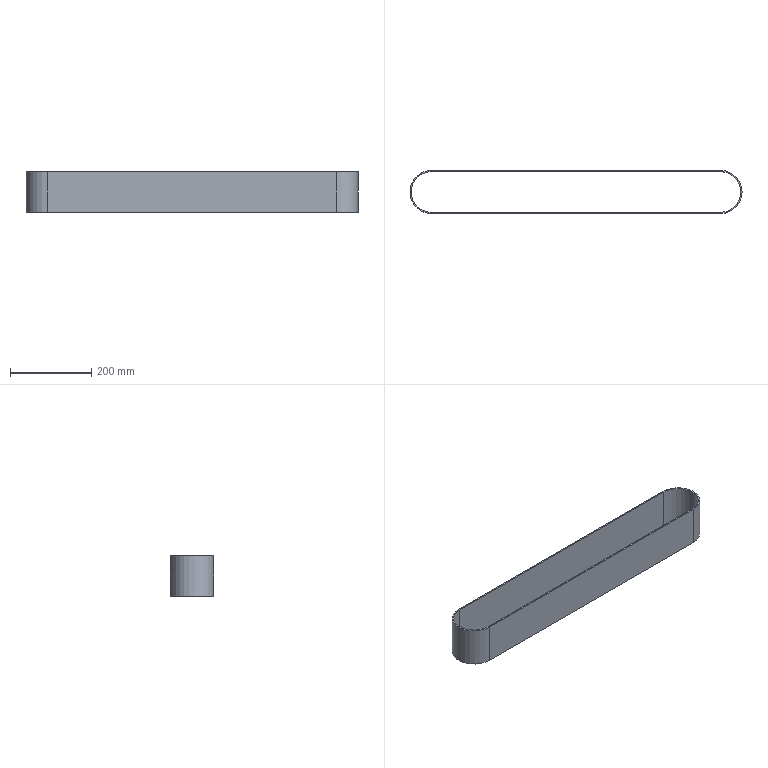Part | STEP file | 1 solid | 12 faces | box 816 x 106 x 100 mm | volume 523075 mm3 | cylinder 6 | plane 6 | commonest cylinder face diameters 100 x3 106 x3
STEP:
#1=CARTESIAN_POINT('',(0.,0.,0.));
#2=DIRECTION('',(0.,0.,1.));
#3=DIRECTION('',(1.,0.,0.));
#4=AXIS2_PLACEMENT_3D('',#1,#2,#3);
#5=CARTESIAN_POINT('',(550.53,56.408,0.));
#6=VERTEX_POINT('',#5);
#7=CARTESIAN_POINT('',(550.53,56.408,100.));
#8=VERTEX_POINT('',#7);
#9=CARTESIAN_POINT('',(550.53,56.408,0.));
#10=DIRECTION('',(0.,0.,1.));
#11=VECTOR('',#10,1.);
#12=LINE('',#9,#11);
#13=CARTESIAN_POINT('',(550.53,6.408,0.));
#14=DIRECTION('',(0.,0.,1.));
#15=DIRECTION('',(1.,0.,0.));
#16=AXIS2_PLACEMENT_3D('',#13,#14,#15);
#17=CYLINDRICAL_SURFACE('',#16,50.);
#18=CARTESIAN_POINT('',(1.571,0.));
#19=DIRECTION('',(0.,1.));
#20=VECTOR('',#19,1.);
#21=LINE('',#18,#20);
#22=(GEOMETRIC_REPRESENTATION_CONTEXT(2)PARAMETRIC_REPRESENTATION_CONTEXT()REPRESENTATION_CONTEXT('',''));
#23=DEFINITIONAL_REPRESENTATION('',(#21),#22);
#24=PCURVE('',#17,#23);
#25=CARTESIAN_POINT('',(550.53,56.408,0.));
#26=DIRECTION('',(0.,1.,0.));
#27=DIRECTION('',(-1.,0.,0.));
#28=AXIS2_PLACEMENT_3D('',#25,#26,#27);
#29=PLANE('',#28);
#30=CARTESIAN_POINT('',(0.,0.));
#31=DIRECTION('',(0.,1.));
#32=VECTOR('',#31,1.);
#33=LINE('',#30,#32);
#34=(GEOMETRIC_REPRESENTATION_CONTEXT(2)PARAMETRIC_REPRESENTATION_CONTEXT()REPRESENTATION_CONTEXT('',''));
#35=DEFINITIONAL_REPRESENTATION('',(#33),#34);
#36=PCURVE('',#29,#35);
#37=SURFACE_CURVE('',#12,(#24,#36),.PCURVE_S1.);
#38=EDGE_CURVE('',#6,#8,#37,.T.);
#39=ORIENTED_EDGE('',*,*,#38,.T.);
#40=CARTESIAN_POINT('',(600.53,6.408,100.));
#41=VERTEX_POINT('',#40);
#42=CARTESIAN_POINT('',(550.53,6.408,100.));
#43=DIRECTION('',(0.,0.,-1.));
#44=DIRECTION('',(1.,0.,0.));
#45=AXIS2_PLACEMENT_3D('',#42,#43,#44);
#46=CIRCLE('',#45,50.);
#47=CARTESIAN_POINT('',(6.283,100.));
#48=DIRECTION('',(-1.,0.));
#49=VECTOR('',#48,1.);
#50=LINE('',#47,#49);
#51=(GEOMETRIC_REPRESENTATION_CONTEXT(2)PARAMETRIC_REPRESENTATION_CONTEXT()REPRESENTATION_CONTEXT('',''));
#52=DEFINITIONAL_REPRESENTATION('',(#50),#51);
#53=PCURVE('',#17,#52);
#54=CARTESIAN_POINT('',(195.531,6.408,100.));
#55=DIRECTION('',(0.,0.,1.));
#56=DIRECTION('',(1.,0.,0.));
#57=AXIS2_PLACEMENT_3D('',#54,#55,#56);
#58=PLANE('',#57);
#59=CARTESIAN_POINT('',(405.,0.));
#60=CARTESIAN_POINT('',(405.,-86.603));
#61=CARTESIAN_POINT('',(330.,-43.301));
#62=CARTESIAN_POINT('',(255.,0.));
#63=CARTESIAN_POINT('',(330.,43.301));
#64=CARTESIAN_POINT('',(405.,86.603));
#65=CARTESIAN_POINT('',(405.,0.));
#66=(BOUNDED_CURVE()B_SPLINE_CURVE(2,(#59,#60,#61,#62,#63,#64,#65),.UNSPECIFIED.,.T.,.F.)B_SPLINE_CURVE_WITH_KNOTS((1,2,2,2,2,1),(-2.094,0.,2.094,4.189,6.283,8.378),.UNSPECIFIED.)CURVE()GEOMETRIC_REPRESENTATION_ITEM()RATIONAL_B_SPLINE_CURVE((1.,0.5,1.,0.5,1.,0.5,1.))REPRESENTATION_ITEM(''));
#67=(GEOMETRIC_REPRESENTATION_CONTEXT(2)PARAMETRIC_REPRESENTATION_CONTEXT()REPRESENTATION_CONTEXT('',''));
#68=DEFINITIONAL_REPRESENTATION('',(#66),#67);
#69=PCURVE('',#58,#68);
#70=SURFACE_CURVE('',#46,(#53,#69),.PCURVE_S1.);
#71=EDGE_CURVE('',#8,#41,#70,.T.);
#72=ORIENTED_EDGE('',*,*,#71,.T.);
#73=CARTESIAN_POINT('',(600.53,6.408,0.));
#74=VERTEX_POINT('',#73);
#75=CARTESIAN_POINT('',(600.53,6.408,0.));
#76=DIRECTION('',(0.,0.,1.));
#77=VECTOR('',#76,1.);
#78=LINE('',#75,#77);
#79=CARTESIAN_POINT('',(0.,0.));
#80=DIRECTION('',(0.,1.));
#81=VECTOR('',#80,1.);
#82=LINE('',#79,#81);
#83=(GEOMETRIC_REPRESENTATION_CONTEXT(2)PARAMETRIC_REPRESENTATION_CONTEXT()REPRESENTATION_CONTEXT('',''));
#84=DEFINITIONAL_REPRESENTATION('',(#82),#83);
#85=PCURVE('',#17,#84);
#86=CARTESIAN_POINT('',(550.53,6.408,0.));
#87=DIRECTION('',(0.,0.,1.));
#88=DIRECTION('',(1.,0.,0.));
#89=AXIS2_PLACEMENT_3D('',#86,#87,#88);
#90=CYLINDRICAL_SURFACE('',#89,50.);
#91=CARTESIAN_POINT('',(6.283,0.));
#92=DIRECTION('',(0.,1.));
#93=VECTOR('',#92,1.);
#94=LINE('',#91,#93);
#95=(GEOMETRIC_REPRESENTATION_CONTEXT(2)PARAMETRIC_REPRESENTATION_CONTEXT()REPRESENTATION_CONTEXT('',''));
#96=DEFINITIONAL_REPRESENTATION('',(#94),#95);
#97=PCURVE('',#90,#96);
#98=SURFACE_CURVE('',#78,(#85,#97),.PCURVE_S1.);
#99=EDGE_CURVE('',#74,#41,#98,.T.);
#100=ORIENTED_EDGE('',*,*,#99,.F.);
#101=CARTESIAN_POINT('',(550.53,6.408,0.));
#102=DIRECTION('',(0.,0.,-1.));
#103=DIRECTION('',(1.,0.,0.));
#104=AXIS2_PLACEMENT_3D('',#101,#102,#103);
#105=CIRCLE('',#104,50.);
#106=CARTESIAN_POINT('',(6.283,0.));
#107=DIRECTION('',(-1.,0.));
#108=VECTOR('',#107,1.);
#109=LINE('',#106,#108);
#110=(GEOMETRIC_REPRESENTATION_CONTEXT(2)PARAMETRIC_REPRESENTATION_CONTEXT()REPRESENTATION_CONTEXT('',''));
#111=DEFINITIONAL_REPRESENTATION('',(#109),#110);
#112=PCURVE('',#17,#111);
#113=CARTESIAN_POINT('',(195.531,6.408,0.));
#114=DIRECTION('',(0.,0.,1.));
#115=DIRECTION('',(1.,0.,0.));
#116=AXIS2_PLACEMENT_3D('',#113,#114,#115);
#117=PLANE('',#116);
#118=CARTESIAN_POINT('',(405.,0.));
#119=CARTESIAN_POINT('',(405.,-86.603));
#120=CARTESIAN_POINT('',(330.,-43.301));
#121=CARTESIAN_POINT('',(255.,0.));
#122=CARTESIAN_POINT('',(330.,43.301));
#123=CARTESIAN_POINT('',(405.,86.603));
#124=CARTESIAN_POINT('',(405.,0.));
#125=(BOUNDED_CURVE()B_SPLINE_CURVE(2,(#118,#119,#120,#121,#122,#123,#124),.UNSPECIFIED.,.T.,.F.)B_SPLINE_CURVE_WITH_KNOTS((1,2,2,2,2,1),(-2.094,0.,2.094,4.189,6.283,8.378),.UNSPECIFIED.)CURVE()GEOMETRIC_REPRESENTATION_ITEM()RATIONAL_B_SPLINE_CURVE((1.,0.5,1.,0.5,1.,0.5,1.))REPRESENTATION_ITEM(''));
#126=(GEOMETRIC_REPRESENTATION_CONTEXT(2)PARAMETRIC_REPRESENTATION_CONTEXT()REPRESENTATION_CONTEXT('',''));
#127=DEFINITIONAL_REPRESENTATION('',(#125),#126);
#128=PCURVE('',#117,#127);
#129=SURFACE_CURVE('',#105,(#112,#128),.PCURVE_S1.);
#130=EDGE_CURVE('',#6,#74,#129,.T.);
#131=ORIENTED_EDGE('',*,*,#130,.F.);
#132=EDGE_LOOP('',(#39,#72,#100,#131));
#133=FACE_BOUND('',#132,.F.);
#134=ADVANCED_FACE('',(#133),#17,.F.);
#135=CARTESIAN_POINT('',(550.53,-46.592,0.));
#136=VERTEX_POINT('',#135);
#137=CARTESIAN_POINT('',(603.53,6.408,0.));
#138=VERTEX_POINT('',#137);
#139=CARTESIAN_POINT('',(550.53,6.408,0.));
#140=DIRECTION('',(0.,0.,1.));
#141=DIRECTION('',(1.,0.,0.));
#142=AXIS2_PLACEMENT_3D('',#139,#140,#141);
#143=CIRCLE('',#142,53.);
#144=CARTESIAN_POINT('',(550.53,6.408,0.));
#145=DIRECTION('',(0.,0.,1.));
#146=DIRECTION('',(1.,0.,0.));
#147=AXIS2_PLACEMENT_3D('',#144,#145,#146);
#148=CYLINDRICAL_SURFACE('',#147,53.);
#149=CARTESIAN_POINT('',(0.,0.));
#150=DIRECTION('',(1.,0.));
#151=VECTOR('',#150,1.);
#152=LINE('',#149,#151);
#153=(GEOMETRIC_REPRESENTATION_CONTEXT(2)PARAMETRIC_REPRESENTATION_CONTEXT()REPRESENTATION_CONTEXT('',''));
#154=DEFINITIONAL_REPRESENTATION('',(#152),#153);
#155=PCURVE('',#148,#154);
#156=CARTESIAN_POINT('',(355.,0.));
#157=DIRECTION('',(1.,0.));
#158=AXIS2_PLACEMENT_2D('',#156,#157);
#159=CIRCLE('',#158,53.);
#160=(GEOMETRIC_REPRESENTATION_CONTEXT(2)PARAMETRIC_REPRESENTATION_CONTEXT()REPRESENTATION_CONTEXT('',''));
#161=DEFINITIONAL_REPRESENTATION('',(#159),#160);
#162=PCURVE('',#117,#161);
#163=SURFACE_CURVE('',#143,(#155,#162),.PCURVE_S1.);
#164=EDGE_CURVE('',#136,#138,#163,.T.);
#165=ORIENTED_EDGE('',*,*,#164,.T.);
#166=CARTESIAN_POINT('',(603.53,6.408,100.));
#167=VERTEX_POINT('',#166);
#168=CARTESIAN_POINT('',(603.53,6.408,0.));
#169=DIRECTION('',(0.,0.,1.));
#170=VECTOR('',#169,1.);
#171=LINE('',#168,#170);
#172=CARTESIAN_POINT('',(6.283,0.));
#173=DIRECTION('',(0.,1.));
#174=VECTOR('',#173,1.);
#175=LINE('',#172,#174);
#176=(GEOMETRIC_REPRESENTATION_CONTEXT(2)PARAMETRIC_REPRESENTATION_CONTEXT()REPRESENTATION_CONTEXT('',''));
#177=DEFINITIONAL_REPRESENTATION('',(#175),#176);
#178=PCURVE('',#148,#177);
#179=CARTESIAN_POINT('',(550.53,6.408,0.));
#180=DIRECTION('',(0.,0.,1.));
#181=DIRECTION('',(1.,0.,0.));
#182=AXIS2_PLACEMENT_3D('',#179,#180,#181);
#183=CYLINDRICAL_SURFACE('',#182,53.);
#184=CARTESIAN_POINT('',(0.,0.));
#185=DIRECTION('',(0.,1.));
#186=VECTOR('',#185,1.);
#187=LINE('',#184,#186);
#188=(GEOMETRIC_REPRESENTATION_CONTEXT(2)PARAMETRIC_REPRESENTATION_CONTEXT()REPRESENTATION_CONTEXT('',''));
#189=DEFINITIONAL_REPRESENTATION('',(#187),#188);
#190=PCURVE('',#183,#189);
#191=SURFACE_CURVE('',#171,(#178,#190),.PCURVE_S1.);
#192=EDGE_CURVE('',#138,#167,#191,.T.);
#193=ORIENTED_EDGE('',*,*,#192,.T.);
#194=CARTESIAN_POINT('',(550.53,-46.592,100.));
#195=VERTEX_POINT('',#194);
#196=CARTESIAN_POINT('',(550.53,6.408,100.));
#197=DIRECTION('',(0.,0.,1.));
#198=DIRECTION('',(1.,0.,0.));
#199=AXIS2_PLACEMENT_3D('',#196,#197,#198);
#200=CIRCLE('',#199,53.);
#201=CARTESIAN_POINT('',(0.,100.));
#202=DIRECTION('',(1.,0.));
#203=VECTOR('',#202,1.);
#204=LINE('',#201,#203);
#205=(GEOMETRIC_REPRESENTATION_CONTEXT(2)PARAMETRIC_REPRESENTATION_CONTEXT()REPRESENTATION_CONTEXT('',''));
#206=DEFINITIONAL_REPRESENTATION('',(#204),#205);
#207=PCURVE('',#148,#206);
#208=CARTESIAN_POINT('',(355.,0.));
#209=DIRECTION('',(1.,0.));
#210=AXIS2_PLACEMENT_2D('',#208,#209);
#211=CIRCLE('',#210,53.);
#212=(GEOMETRIC_REPRESENTATION_CONTEXT(2)PARAMETRIC_REPRESENTATION_CONTEXT()REPRESENTATION_CONTEXT('',''));
#213=DEFINITIONAL_REPRESENTATION('',(#211),#212);
#214=PCURVE('',#58,#213);
#215=SURFACE_CURVE('',#200,(#207,#214),.PCURVE_S1.);
#216=EDGE_CURVE('',#195,#167,#215,.T.);
#217=ORIENTED_EDGE('',*,*,#216,.F.);
#218=CARTESIAN_POINT('',(550.53,-46.592,0.));
#219=DIRECTION('',(0.,0.,-1.));
#220=VECTOR('',#219,1.);
#221=LINE('',#218,#220);
#222=CARTESIAN_POINT('',(4.712,0.));
#223=DIRECTION('',(0.,-1.));
#224=VECTOR('',#223,1.);
#225=LINE('',#222,#224);
#226=(GEOMETRIC_REPRESENTATION_CONTEXT(2)PARAMETRIC_REPRESENTATION_CONTEXT()REPRESENTATION_CONTEXT('',''));
#227=DEFINITIONAL_REPRESENTATION('',(#225),#226);
#228=PCURVE('',#148,#227);
#229=CARTESIAN_POINT('',(-159.47,-46.592,0.));
#230=DIRECTION('',(0.,-1.,0.));
#231=DIRECTION('',(1.,0.,0.));
#232=AXIS2_PLACEMENT_3D('',#229,#230,#231);
#233=PLANE('',#232);
#234=CARTESIAN_POINT('',(710.,0.));
#235=DIRECTION('',(0.,-1.));
#236=VECTOR('',#235,1.);
#237=LINE('',#234,#236);
#238=(GEOMETRIC_REPRESENTATION_CONTEXT(2)PARAMETRIC_REPRESENTATION_CONTEXT()REPRESENTATION_CONTEXT('',''));
#239=DEFINITIONAL_REPRESENTATION('',(#237),#238);
#240=PCURVE('',#233,#239);
#241=SURFACE_CURVE('',#221,(#228,#240),.PCURVE_S1.);
#242=EDGE_CURVE('',#195,#136,#241,.T.);
#243=ORIENTED_EDGE('',*,*,#242,.T.);
#244=EDGE_LOOP('',(#165,#193,#217,#243));
#245=FACE_BOUND('',#244,.T.);
#246=ADVANCED_FACE('',(#245),#148,.T.);
#247=CARTESIAN_POINT('',(-159.47,-43.592,100.));
#248=VERTEX_POINT('',#247);
#249=CARTESIAN_POINT('',(-159.47,-43.592,0.));
#250=VERTEX_POINT('',#249);
#251=CARTESIAN_POINT('',(-159.47,-43.592,0.));
#252=DIRECTION('',(0.,0.,-1.));
#253=VECTOR('',#252,1.);
#254=LINE('',#251,#253);
#255=CARTESIAN_POINT('',(-159.47,-43.592,0.));
#256=DIRECTION('',(0.,-1.,0.));
#257=DIRECTION('',(1.,0.,0.));
#258=AXIS2_PLACEMENT_3D('',#255,#256,#257);
#259=PLANE('',#258);
#260=CARTESIAN_POINT('',(0.,0.));
#261=DIRECTION('',(0.,-1.));
#262=VECTOR('',#261,1.);
#263=LINE('',#260,#262);
#264=(GEOMETRIC_REPRESENTATION_CONTEXT(2)PARAMETRIC_REPRESENTATION_CONTEXT()REPRESENTATION_CONTEXT('',''));
#265=DEFINITIONAL_REPRESENTATION('',(#263),#264);
#266=PCURVE('',#259,#265);
#267=CARTESIAN_POINT('',(-159.47,6.408,0.));
#268=DIRECTION('',(0.,0.,1.));
#269=DIRECTION('',(1.,0.,0.));
#270=AXIS2_PLACEMENT_3D('',#267,#268,#269);
#271=CYLINDRICAL_SURFACE('',#270,50.);
#272=CARTESIAN_POINT('',(4.712,0.));
#273=DIRECTION('',(0.,-1.));
#274=VECTOR('',#273,1.);
#275=LINE('',#272,#274);
#276=(GEOMETRIC_REPRESENTATION_CONTEXT(2)PARAMETRIC_REPRESENTATION_CONTEXT()REPRESENTATION_CONTEXT('',''));
#277=DEFINITIONAL_REPRESENTATION('',(#275),#276);
#278=PCURVE('',#271,#277);
#279=SURFACE_CURVE('',#254,(#266,#278),.PCURVE_S1.);
#280=EDGE_CURVE('',#248,#250,#279,.T.);
#281=ORIENTED_EDGE('',*,*,#280,.F.);
#282=CARTESIAN_POINT('',(550.53,-43.592,100.));
#283=VERTEX_POINT('',#282);
#284=CARTESIAN_POINT('',(-159.47,-43.592,100.));
#285=DIRECTION('',(-1.,0.,0.));
#286=VECTOR('',#285,1.);
#287=LINE('',#284,#286);
#288=CARTESIAN_POINT('',(0.,100.));
#289=DIRECTION('',(-1.,0.));
#290=VECTOR('',#289,1.);
#291=LINE('',#288,#290);
#292=(GEOMETRIC_REPRESENTATION_CONTEXT(2)PARAMETRIC_REPRESENTATION_CONTEXT()REPRESENTATION_CONTEXT('',''));
#293=DEFINITIONAL_REPRESENTATION('',(#291),#292);
#294=PCURVE('',#259,#293);
#295=CARTESIAN_POINT('',(-355.,-50.));
#296=DIRECTION('',(-1.,0.));
#297=VECTOR('',#296,1.);
#298=LINE('',#295,#297);
#299=(GEOMETRIC_REPRESENTATION_CONTEXT(2)PARAMETRIC_REPRESENTATION_CONTEXT()REPRESENTATION_CONTEXT('',''));
#300=DEFINITIONAL_REPRESENTATION('',(#298),#299);
#301=PCURVE('',#58,#300);
#302=SURFACE_CURVE('',#287,(#294,#301),.PCURVE_S1.);
#303=EDGE_CURVE('',#283,#248,#302,.T.);
#304=ORIENTED_EDGE('',*,*,#303,.F.);
#305=CARTESIAN_POINT('',(550.53,-43.592,0.));
#306=VERTEX_POINT('',#305);
#307=CARTESIAN_POINT('',(550.53,-43.592,0.));
#308=DIRECTION('',(0.,0.,1.));
#309=VECTOR('',#308,1.);
#310=LINE('',#307,#309);
#311=CARTESIAN_POINT('',(710.,0.));
#312=DIRECTION('',(0.,1.));
#313=VECTOR('',#312,1.);
#314=LINE('',#311,#313);
#315=(GEOMETRIC_REPRESENTATION_CONTEXT(2)PARAMETRIC_REPRESENTATION_CONTEXT()REPRESENTATION_CONTEXT('',''));
#316=DEFINITIONAL_REPRESENTATION('',(#314),#315);
#317=PCURVE('',#259,#316);
#318=CARTESIAN_POINT('',(4.712,0.));
#319=DIRECTION('',(0.,1.));
#320=VECTOR('',#319,1.);
#321=LINE('',#318,#320);
#322=(GEOMETRIC_REPRESENTATION_CONTEXT(2)PARAMETRIC_REPRESENTATION_CONTEXT()REPRESENTATION_CONTEXT('',''));
#323=DEFINITIONAL_REPRESENTATION('',(#321),#322);
#324=PCURVE('',#90,#323);
#325=SURFACE_CURVE('',#310,(#317,#324),.PCURVE_S1.);
#326=EDGE_CURVE('',#306,#283,#325,.T.);
#327=ORIENTED_EDGE('',*,*,#326,.F.);
#328=CARTESIAN_POINT('',(-159.47,-43.592,0.));
#329=DIRECTION('',(1.,0.,0.));
#330=VECTOR('',#329,1.);
#331=LINE('',#328,#330);
#332=CARTESIAN_POINT('',(0.,0.));
#333=DIRECTION('',(1.,0.));
#334=VECTOR('',#333,1.);
#335=LINE('',#332,#334);
#336=(GEOMETRIC_REPRESENTATION_CONTEXT(2)PARAMETRIC_REPRESENTATION_CONTEXT()REPRESENTATION_CONTEXT('',''));
#337=DEFINITIONAL_REPRESENTATION('',(#335),#336);
#338=PCURVE('',#259,#337);
#339=CARTESIAN_POINT('',(-355.,-50.));
#340=DIRECTION('',(1.,0.));
#341=VECTOR('',#340,1.);
#342=LINE('',#339,#341);
#343=(GEOMETRIC_REPRESENTATION_CONTEXT(2)PARAMETRIC_REPRESENTATION_CONTEXT()REPRESENTATION_CONTEXT('',''));
#344=DEFINITIONAL_REPRESENTATION('',(#342),#343);
#345=PCURVE('',#117,#344);
#346=SURFACE_CURVE('',#331,(#338,#345),.PCURVE_S1.);
#347=EDGE_CURVE('',#250,#306,#346,.T.);
#348=ORIENTED_EDGE('',*,*,#347,.F.);
#349=EDGE_LOOP('',(#281,#304,#327,#348));
#350=FACE_BOUND('',#349,.T.);
#351=ADVANCED_FACE('',(#350),#259,.F.);
#352=ORIENTED_EDGE('',*,*,#164,.F.);
#353=CARTESIAN_POINT('',(-159.47,-46.592,0.));
#354=VERTEX_POINT('',#353);
#355=CARTESIAN_POINT('',(195.531,-46.592,0.));
#356=DIRECTION('',(1.,0.,0.));
#357=VECTOR('',#356,1.);
#358=LINE('',#355,#357);
#359=CARTESIAN_POINT('',(0.,-53.));
#360=DIRECTION('',(1.,0.));
#361=VECTOR('',#360,1.);
#362=LINE('',#359,#361);
#363=(GEOMETRIC_REPRESENTATION_CONTEXT(2)PARAMETRIC_REPRESENTATION_CONTEXT()REPRESENTATION_CONTEXT('',''));
#364=DEFINITIONAL_REPRESENTATION('',(#362),#363);
#365=PCURVE('',#117,#364);
#366=CARTESIAN_POINT('',(355.,0.));
#367=DIRECTION('',(1.,0.));
#368=VECTOR('',#367,1.);
#369=LINE('',#366,#368);
#370=(GEOMETRIC_REPRESENTATION_CONTEXT(2)PARAMETRIC_REPRESENTATION_CONTEXT()REPRESENTATION_CONTEXT('',''));
#371=DEFINITIONAL_REPRESENTATION('',(#369),#370);
#372=PCURVE('',#233,#371);
#373=SURFACE_CURVE('',#358,(#365,#372),.PCURVE_S1.);
#374=EDGE_CURVE('',#354,#136,#373,.T.);
#375=ORIENTED_EDGE('',*,*,#374,.F.);
#376=CARTESIAN_POINT('',(-159.47,59.408,0.));
#377=VERTEX_POINT('',#376);
#378=CARTESIAN_POINT('',(-159.47,6.408,0.));
#379=DIRECTION('',(0.,0.,1.));
#380=DIRECTION('',(1.,0.,0.));
#381=AXIS2_PLACEMENT_3D('',#378,#379,#380);
#382=CIRCLE('',#381,53.);
#383=CARTESIAN_POINT('',(-355.,0.));
#384=DIRECTION('',(1.,0.));
#385=AXIS2_PLACEMENT_2D('',#383,#384);
#386=CIRCLE('',#385,53.);
#387=(GEOMETRIC_REPRESENTATION_CONTEXT(2)PARAMETRIC_REPRESENTATION_CONTEXT()REPRESENTATION_CONTEXT('',''));
#388=DEFINITIONAL_REPRESENTATION('',(#386),#387);
#389=PCURVE('',#117,#388);
#390=CARTESIAN_POINT('',(-159.47,6.408,0.));
#391=DIRECTION('',(0.,0.,1.));
#392=DIRECTION('',(1.,0.,0.));
#393=AXIS2_PLACEMENT_3D('',#390,#391,#392);
#394=CYLINDRICAL_SURFACE('',#393,53.);
#395=CARTESIAN_POINT('',(0.,0.));
#396=DIRECTION('',(1.,0.));
#397=VECTOR('',#396,1.);
#398=LINE('',#395,#397);
#399=(GEOMETRIC_REPRESENTATION_CONTEXT(2)PARAMETRIC_REPRESENTATION_CONTEXT()REPRESENTATION_CONTEXT('',''));
#400=DEFINITIONAL_REPRESENTATION('',(#398),#399);
#401=PCURVE('',#394,#400);
#402=SURFACE_CURVE('',#382,(#389,#401),.PCURVE_S1.);
#403=EDGE_CURVE('',#377,#354,#402,.T.);
#404=ORIENTED_EDGE('',*,*,#403,.F.);
#405=CARTESIAN_POINT('',(550.53,59.408,0.));
#406=VERTEX_POINT('',#405);
#407=CARTESIAN_POINT('',(195.531,59.408,0.));
#408=DIRECTION('',(-1.,0.,0.));
#409=VECTOR('',#408,1.);
#410=LINE('',#407,#409);
#411=CARTESIAN_POINT('',(0.,53.));
#412=DIRECTION('',(-1.,0.));
#413=VECTOR('',#412,1.);
#414=LINE('',#411,#413);
#415=(GEOMETRIC_REPRESENTATION_CONTEXT(2)PARAMETRIC_REPRESENTATION_CONTEXT()REPRESENTATION_CONTEXT('',''));
#416=DEFINITIONAL_REPRESENTATION('',(#414),#415);
#417=PCURVE('',#117,#416);
#418=CARTESIAN_POINT('',(550.53,59.408,0.));
#419=DIRECTION('',(0.,1.,0.));
#420=DIRECTION('',(-1.,0.,0.));
#421=AXIS2_PLACEMENT_3D('',#418,#419,#420);
#422=PLANE('',#421);
#423=CARTESIAN_POINT('',(355.,0.));
#424=DIRECTION('',(1.,0.));
#425=VECTOR('',#424,1.);
#426=LINE('',#423,#425);
#427=(GEOMETRIC_REPRESENTATION_CONTEXT(2)PARAMETRIC_REPRESENTATION_CONTEXT()REPRESENTATION_CONTEXT('',''));
#428=DEFINITIONAL_REPRESENTATION('',(#426),#427);
#429=PCURVE('',#422,#428);
#430=SURFACE_CURVE('',#410,(#417,#429),.PCURVE_S1.);
#431=EDGE_CURVE('',#406,#377,#430,.T.);
#432=ORIENTED_EDGE('',*,*,#431,.F.);
#433=CARTESIAN_POINT('',(550.53,6.408,0.));
#434=DIRECTION('',(0.,0.,1.));
#435=DIRECTION('',(1.,0.,0.));
#436=AXIS2_PLACEMENT_3D('',#433,#434,#435);
#437=CIRCLE('',#436,53.);
#438=CARTESIAN_POINT('',(355.,0.));
#439=DIRECTION('',(1.,0.));
#440=AXIS2_PLACEMENT_2D('',#438,#439);
#441=CIRCLE('',#440,53.);
#442=(GEOMETRIC_REPRESENTATION_CONTEXT(2)PARAMETRIC_REPRESENTATION_CONTEXT()REPRESENTATION_CONTEXT('',''));
#443=DEFINITIONAL_REPRESENTATION('',(#441),#442);
#444=PCURVE('',#117,#443);
#445=CARTESIAN_POINT('',(0.,0.));
#446=DIRECTION('',(1.,0.));
#447=VECTOR('',#446,1.);
#448=LINE('',#445,#447);
#449=(GEOMETRIC_REPRESENTATION_CONTEXT(2)PARAMETRIC_REPRESENTATION_CONTEXT()REPRESENTATION_CONTEXT('',''));
#450=DEFINITIONAL_REPRESENTATION('',(#448),#449);
#451=PCURVE('',#183,#450);
#452=SURFACE_CURVE('',#437,(#444,#451),.PCURVE_S1.);
#453=EDGE_CURVE('',#138,#406,#452,.T.);
#454=ORIENTED_EDGE('',*,*,#453,.F.);
#455=EDGE_LOOP('',(#352,#375,#404,#432,#454));
#456=FACE_BOUND('',#455,.T.);
#457=CARTESIAN_POINT('',(-159.47,56.408,0.));
#458=VERTEX_POINT('',#457);
#459=CARTESIAN_POINT('',(195.531,56.408,0.));
#460=DIRECTION('',(1.,0.,0.));
#461=VECTOR('',#460,1.);
#462=LINE('',#459,#461);
#463=CARTESIAN_POINT('',(0.,50.));
#464=DIRECTION('',(1.,0.));
#465=VECTOR('',#464,1.);
#466=LINE('',#463,#465);
#467=(GEOMETRIC_REPRESENTATION_CONTEXT(2)PARAMETRIC_REPRESENTATION_CONTEXT()REPRESENTATION_CONTEXT('',''));
#468=DEFINITIONAL_REPRESENTATION('',(#466),#467);
#469=PCURVE('',#117,#468);
#470=CARTESIAN_POINT('',(355.,0.));
#471=DIRECTION('',(-1.,0.));
#472=VECTOR('',#471,1.);
#473=LINE('',#470,#472);
#474=(GEOMETRIC_REPRESENTATION_CONTEXT(2)PARAMETRIC_REPRESENTATION_CONTEXT()REPRESENTATION_CONTEXT('',''));
#475=DEFINITIONAL_REPRESENTATION('',(#473),#474);
#476=PCURVE('',#29,#475);
#477=SURFACE_CURVE('',#462,(#469,#476),.PCURVE_S1.);
#478=EDGE_CURVE('',#458,#6,#477,.T.);
#479=ORIENTED_EDGE('',*,*,#478,.F.);
#480=CARTESIAN_POINT('',(-159.47,6.408,0.));
#481=DIRECTION('',(0.,0.,-1.));
#482=DIRECTION('',(1.,0.,0.));
#483=AXIS2_PLACEMENT_3D('',#480,#481,#482);
#484=CIRCLE('',#483,50.);
#485=CARTESIAN_POINT('',(-305.,0.));
#486=CARTESIAN_POINT('',(-305.,-86.603));
#487=CARTESIAN_POINT('',(-380.,-43.301));
#488=CARTESIAN_POINT('',(-455.,0.));
#489=CARTESIAN_POINT('',(-380.,43.301));
#490=CARTESIAN_POINT('',(-305.,86.603));
#491=CARTESIAN_POINT('',(-305.,0.));
#492=(BOUNDED_CURVE()B_SPLINE_CURVE(2,(#485,#486,#487,#488,#489,#490,#491),.UNSPECIFIED.,.T.,.F.)B_SPLINE_CURVE_WITH_KNOTS((1,2,2,2,2,1),(-2.094,0.,2.094,4.189,6.283,8.378),.UNSPECIFIED.)CURVE()GEOMETRIC_REPRESENTATION_ITEM()RATIONAL_B_SPLINE_CURVE((1.,0.5,1.,0.5,1.,0.5,1.))REPRESENTATION_ITEM(''));
#493=(GEOMETRIC_REPRESENTATION_CONTEXT(2)PARAMETRIC_REPRESENTATION_CONTEXT()REPRESENTATION_CONTEXT('',''));
#494=DEFINITIONAL_REPRESENTATION('',(#492),#493);
#495=PCURVE('',#117,#494);
#496=CARTESIAN_POINT('',(6.283,0.));
#497=DIRECTION('',(-1.,0.));
#498=VECTOR('',#497,1.);
#499=LINE('',#496,#498);
#500=(GEOMETRIC_REPRESENTATION_CONTEXT(2)PARAMETRIC_REPRESENTATION_CONTEXT()REPRESENTATION_CONTEXT('',''));
#501=DEFINITIONAL_REPRESENTATION('',(#499),#500);
#502=PCURVE('',#271,#501);
#503=SURFACE_CURVE('',#484,(#495,#502),.PCURVE_S1.);
#504=EDGE_CURVE('',#250,#458,#503,.T.);
#505=ORIENTED_EDGE('',*,*,#504,.F.);
#506=ORIENTED_EDGE('',*,*,#347,.T.);
#507=CARTESIAN_POINT('',(550.53,6.408,0.));
#508=DIRECTION('',(0.,0.,-1.));
#509=DIRECTION('',(1.,0.,0.));
#510=AXIS2_PLACEMENT_3D('',#507,#508,#509);
#511=CIRCLE('',#510,50.);
#512=CARTESIAN_POINT('',(405.,0.));
#513=CARTESIAN_POINT('',(405.,-86.603));
#514=CARTESIAN_POINT('',(330.,-43.301));
#515=CARTESIAN_POINT('',(255.,0.));
#516=CARTESIAN_POINT('',(330.,43.301));
#517=CARTESIAN_POINT('',(405.,86.603));
#518=CARTESIAN_POINT('',(405.,0.));
#519=(BOUNDED_CURVE()B_SPLINE_CURVE(2,(#512,#513,#514,#515,#516,#517,#518),.UNSPECIFIED.,.T.,.F.)B_SPLINE_CURVE_WITH_KNOTS((1,2,2,2,2,1),(-2.094,0.,2.094,4.189,6.283,8.378),.UNSPECIFIED.)CURVE()GEOMETRIC_REPRESENTATION_ITEM()RATIONAL_B_SPLINE_CURVE((1.,0.5,1.,0.5,1.,0.5,1.))REPRESENTATION_ITEM(''));
#520=(GEOMETRIC_REPRESENTATION_CONTEXT(2)PARAMETRIC_REPRESENTATION_CONTEXT()REPRESENTATION_CONTEXT('',''));
#521=DEFINITIONAL_REPRESENTATION('',(#519),#520);
#522=PCURVE('',#117,#521);
#523=CARTESIAN_POINT('',(6.283,0.));
#524=DIRECTION('',(-1.,0.));
#525=VECTOR('',#524,1.);
#526=LINE('',#523,#525);
#527=(GEOMETRIC_REPRESENTATION_CONTEXT(2)PARAMETRIC_REPRESENTATION_CONTEXT()REPRESENTATION_CONTEXT('',''));
#528=DEFINITIONAL_REPRESENTATION('',(#526),#527);
#529=PCURVE('',#90,#528);
#530=SURFACE_CURVE('',#511,(#522,#529),.PCURVE_S1.);
#531=EDGE_CURVE('',#74,#306,#530,.T.);
#532=ORIENTED_EDGE('',*,*,#531,.F.);
#533=ORIENTED_EDGE('',*,*,#130,.F.);
#534=EDGE_LOOP('',(#479,#505,#506,#532,#533));
#535=FACE_BOUND('',#534,.T.);
#536=ADVANCED_FACE('',(#456,#535),#117,.F.);
#537=ORIENTED_EDGE('',*,*,#504,.F.);
#538=ORIENTED_EDGE('',*,*,#280,.F.);
#539=CARTESIAN_POINT('',(-159.47,56.408,100.));
#540=VERTEX_POINT('',#539);
#541=CARTESIAN_POINT('',(-159.47,6.408,100.));
#542=DIRECTION('',(0.,0.,-1.));
#543=DIRECTION('',(1.,0.,0.));
#544=AXIS2_PLACEMENT_3D('',#541,#542,#543);
#545=CIRCLE('',#544,50.);
#546=CARTESIAN_POINT('',(6.283,100.));
#547=DIRECTION('',(-1.,0.));
#548=VECTOR('',#547,1.);
#549=LINE('',#546,#548);
#550=(GEOMETRIC_REPRESENTATION_CONTEXT(2)PARAMETRIC_REPRESENTATION_CONTEXT()REPRESENTATION_CONTEXT('',''));
#551=DEFINITIONAL_REPRESENTATION('',(#549),#550);
#552=PCURVE('',#271,#551);
#553=CARTESIAN_POINT('',(-305.,0.));
#554=CARTESIAN_POINT('',(-305.,-86.603));
#555=CARTESIAN_POINT('',(-380.,-43.301));
#556=CARTESIAN_POINT('',(-455.,0.));
#557=CARTESIAN_POINT('',(-380.,43.301));
#558=CARTESIAN_POINT('',(-305.,86.603));
#559=CARTESIAN_POINT('',(-305.,0.));
#560=(BOUNDED_CURVE()B_SPLINE_CURVE(2,(#553,#554,#555,#556,#557,#558,#559),.UNSPECIFIED.,.T.,.F.)B_SPLINE_CURVE_WITH_KNOTS((1,2,2,2,2,1),(-2.094,0.,2.094,4.189,6.283,8.378),.UNSPECIFIED.)CURVE()GEOMETRIC_REPRESENTATION_ITEM()RATIONAL_B_SPLINE_CURVE((1.,0.5,1.,0.5,1.,0.5,1.))REPRESENTATION_ITEM(''));
#561=(GEOMETRIC_REPRESENTATION_CONTEXT(2)PARAMETRIC_REPRESENTATION_CONTEXT()REPRESENTATION_CONTEXT('',''));
#562=DEFINITIONAL_REPRESENTATION('',(#560),#561);
#563=PCURVE('',#58,#562);
#564=SURFACE_CURVE('',#545,(#552,#563),.PCURVE_S1.);
#565=EDGE_CURVE('',#248,#540,#564,.T.);
#566=ORIENTED_EDGE('',*,*,#565,.T.);
#567=CARTESIAN_POINT('',(-159.47,56.408,0.));
#568=DIRECTION('',(0.,0.,-1.));
#569=VECTOR('',#568,1.);
#570=LINE('',#567,#569);
#571=CARTESIAN_POINT('',(1.571,0.));
#572=DIRECTION('',(0.,-1.));
#573=VECTOR('',#572,1.);
#574=LINE('',#571,#573);
#575=(GEOMETRIC_REPRESENTATION_CONTEXT(2)PARAMETRIC_REPRESENTATION_CONTEXT()REPRESENTATION_CONTEXT('',''));
#576=DEFINITIONAL_REPRESENTATION('',(#574),#575);
#577=PCURVE('',#271,#576);
#578=CARTESIAN_POINT('',(710.,0.));
#579=DIRECTION('',(0.,-1.));
#580=VECTOR('',#579,1.);
#581=LINE('',#578,#580);
#582=(GEOMETRIC_REPRESENTATION_CONTEXT(2)PARAMETRIC_REPRESENTATION_CONTEXT()REPRESENTATION_CONTEXT('',''));
#583=DEFINITIONAL_REPRESENTATION('',(#581),#582);
#584=PCURVE('',#29,#583);
#585=SURFACE_CURVE('',#570,(#577,#584),.PCURVE_S1.);
#586=EDGE_CURVE('',#540,#458,#585,.T.);
#587=ORIENTED_EDGE('',*,*,#586,.T.);
#588=EDGE_LOOP('',(#537,#538,#566,#587));
#589=FACE_BOUND('',#588,.F.);
#590=ADVANCED_FACE('',(#589),#271,.F.);
#591=CARTESIAN_POINT('',(-159.47,-46.592,100.));
#592=VERTEX_POINT('',#591);
#593=CARTESIAN_POINT('',(195.531,-46.592,100.));
#594=DIRECTION('',(1.,0.,0.));
#595=VECTOR('',#594,1.);
#596=LINE('',#593,#595);
#597=CARTESIAN_POINT('',(0.,-53.));
#598=DIRECTION('',(1.,0.));
#599=VECTOR('',#598,1.);
#600=LINE('',#597,#599);
#601=(GEOMETRIC_REPRESENTATION_CONTEXT(2)PARAMETRIC_REPRESENTATION_CONTEXT()REPRESENTATION_CONTEXT('',''));
#602=DEFINITIONAL_REPRESENTATION('',(#600),#601);
#603=PCURVE('',#58,#602);
#604=CARTESIAN_POINT('',(355.,100.));
#605=DIRECTION('',(1.,0.));
#606=VECTOR('',#605,1.);
#607=LINE('',#604,#606);
#608=(GEOMETRIC_REPRESENTATION_CONTEXT(2)PARAMETRIC_REPRESENTATION_CONTEXT()REPRESENTATION_CONTEXT('',''));
#609=DEFINITIONAL_REPRESENTATION('',(#607),#608);
#610=PCURVE('',#233,#609);
#611=SURFACE_CURVE('',#596,(#603,#610),.PCURVE_S1.);
#612=EDGE_CURVE('',#592,#195,#611,.T.);
#613=ORIENTED_EDGE('',*,*,#612,.T.);
#614=ORIENTED_EDGE('',*,*,#216,.T.);
#615=CARTESIAN_POINT('',(550.53,59.408,100.));
#616=VERTEX_POINT('',#615);
#617=CARTESIAN_POINT('',(550.53,6.408,100.));
#618=DIRECTION('',(0.,0.,1.));
#619=DIRECTION('',(1.,0.,0.));
#620=AXIS2_PLACEMENT_3D('',#617,#618,#619);
#621=CIRCLE('',#620,53.);
#622=CARTESIAN_POINT('',(355.,0.));
#623=DIRECTION('',(1.,0.));
#624=AXIS2_PLACEMENT_2D('',#622,#623);
#625=CIRCLE('',#624,53.);
#626=(GEOMETRIC_REPRESENTATION_CONTEXT(2)PARAMETRIC_REPRESENTATION_CONTEXT()REPRESENTATION_CONTEXT('',''));
#627=DEFINITIONAL_REPRESENTATION('',(#625),#626);
#628=PCURVE('',#58,#627);
#629=CARTESIAN_POINT('',(0.,100.));
#630=DIRECTION('',(1.,0.));
#631=VECTOR('',#630,1.);
#632=LINE('',#629,#631);
#633=(GEOMETRIC_REPRESENTATION_CONTEXT(2)PARAMETRIC_REPRESENTATION_CONTEXT()REPRESENTATION_CONTEXT('',''));
#634=DEFINITIONAL_REPRESENTATION('',(#632),#633);
#635=PCURVE('',#183,#634);
#636=SURFACE_CURVE('',#621,(#628,#635),.PCURVE_S1.);
#637=EDGE_CURVE('',#167,#616,#636,.T.);
#638=ORIENTED_EDGE('',*,*,#637,.T.);
#639=CARTESIAN_POINT('',(-159.47,59.408,100.));
#640=VERTEX_POINT('',#639);
#641=CARTESIAN_POINT('',(195.531,59.408,100.));
#642=DIRECTION('',(-1.,0.,0.));
#643=VECTOR('',#642,1.);
#644=LINE('',#641,#643);
#645=CARTESIAN_POINT('',(0.,53.));
#646=DIRECTION('',(-1.,0.));
#647=VECTOR('',#646,1.);
#648=LINE('',#645,#647);
#649=(GEOMETRIC_REPRESENTATION_CONTEXT(2)PARAMETRIC_REPRESENTATION_CONTEXT()REPRESENTATION_CONTEXT('',''));
#650=DEFINITIONAL_REPRESENTATION('',(#648),#649);
#651=PCURVE('',#58,#650);
#652=CARTESIAN_POINT('',(355.,100.));
#653=DIRECTION('',(1.,0.));
#654=VECTOR('',#653,1.);
#655=LINE('',#652,#654);
#656=(GEOMETRIC_REPRESENTATION_CONTEXT(2)PARAMETRIC_REPRESENTATION_CONTEXT()REPRESENTATION_CONTEXT('',''));
#657=DEFINITIONAL_REPRESENTATION('',(#655),#656);
#658=PCURVE('',#422,#657);
#659=SURFACE_CURVE('',#644,(#651,#658),.PCURVE_S1.);
#660=EDGE_CURVE('',#616,#640,#659,.T.);
#661=ORIENTED_EDGE('',*,*,#660,.T.);
#662=CARTESIAN_POINT('',(-159.47,6.408,100.));
#663=DIRECTION('',(0.,0.,1.));
#664=DIRECTION('',(1.,0.,0.));
#665=AXIS2_PLACEMENT_3D('',#662,#663,#664);
#666=CIRCLE('',#665,53.);
#667=CARTESIAN_POINT('',(-355.,0.));
#668=DIRECTION('',(1.,0.));
#669=AXIS2_PLACEMENT_2D('',#667,#668);
#670=CIRCLE('',#669,53.);
#671=(GEOMETRIC_REPRESENTATION_CONTEXT(2)PARAMETRIC_REPRESENTATION_CONTEXT()REPRESENTATION_CONTEXT('',''));
#672=DEFINITIONAL_REPRESENTATION('',(#670),#671);
#673=PCURVE('',#58,#672);
#674=CARTESIAN_POINT('',(0.,100.));
#675=DIRECTION('',(1.,0.));
#676=VECTOR('',#675,1.);
#677=LINE('',#674,#676);
#678=(GEOMETRIC_REPRESENTATION_CONTEXT(2)PARAMETRIC_REPRESENTATION_CONTEXT()REPRESENTATION_CONTEXT('',''));
#679=DEFINITIONAL_REPRESENTATION('',(#677),#678);
#680=PCURVE('',#394,#679);
#681=SURFACE_CURVE('',#666,(#673,#680),.PCURVE_S1.);
#682=EDGE_CURVE('',#640,#592,#681,.T.);
#683=ORIENTED_EDGE('',*,*,#682,.T.);
#684=EDGE_LOOP('',(#613,#614,#638,#661,#683));
#685=FACE_BOUND('',#684,.T.);
#686=ORIENTED_EDGE('',*,*,#565,.T.);
#687=CARTESIAN_POINT('',(195.531,56.408,100.));
#688=DIRECTION('',(1.,0.,0.));
#689=VECTOR('',#688,1.);
#690=LINE('',#687,#689);
#691=CARTESIAN_POINT('',(0.,50.));
#692=DIRECTION('',(1.,0.));
#693=VECTOR('',#692,1.);
#694=LINE('',#691,#693);
#695=(GEOMETRIC_REPRESENTATION_CONTEXT(2)PARAMETRIC_REPRESENTATION_CONTEXT()REPRESENTATION_CONTEXT('',''));
#696=DEFINITIONAL_REPRESENTATION('',(#694),#695);
#697=PCURVE('',#58,#696);
#698=CARTESIAN_POINT('',(355.,100.));
#699=DIRECTION('',(-1.,0.));
#700=VECTOR('',#699,1.);
#701=LINE('',#698,#700);
#702=(GEOMETRIC_REPRESENTATION_CONTEXT(2)PARAMETRIC_REPRESENTATION_CONTEXT()REPRESENTATION_CONTEXT('',''));
#703=DEFINITIONAL_REPRESENTATION('',(#701),#702);
#704=PCURVE('',#29,#703);
#705=SURFACE_CURVE('',#690,(#697,#704),.PCURVE_S1.);
#706=EDGE_CURVE('',#540,#8,#705,.T.);
#707=ORIENTED_EDGE('',*,*,#706,.T.);
#708=ORIENTED_EDGE('',*,*,#71,.T.);
#709=CARTESIAN_POINT('',(550.53,6.408,100.));
#710=DIRECTION('',(0.,0.,-1.));
#711=DIRECTION('',(1.,0.,0.));
#712=AXIS2_PLACEMENT_3D('',#709,#710,#711);
#713=CIRCLE('',#712,50.);
#714=CARTESIAN_POINT('',(405.,0.));
#715=CARTESIAN_POINT('',(405.,-86.603));
#716=CARTESIAN_POINT('',(330.,-43.301));
#717=CARTESIAN_POINT('',(255.,0.));
#718=CARTESIAN_POINT('',(330.,43.301));
#719=CARTESIAN_POINT('',(405.,86.603));
#720=CARTESIAN_POINT('',(405.,0.));
#721=(BOUNDED_CURVE()B_SPLINE_CURVE(2,(#714,#715,#716,#717,#718,#719,#720),.UNSPECIFIED.,.T.,.F.)B_SPLINE_CURVE_WITH_KNOTS((1,2,2,2,2,1),(-2.094,0.,2.094,4.189,6.283,8.378),.UNSPECIFIED.)CURVE()GEOMETRIC_REPRESENTATION_ITEM()RATIONAL_B_SPLINE_CURVE((1.,0.5,1.,0.5,1.,0.5,1.))REPRESENTATION_ITEM(''));
#722=(GEOMETRIC_REPRESENTATION_CONTEXT(2)PARAMETRIC_REPRESENTATION_CONTEXT()REPRESENTATION_CONTEXT('',''));
#723=DEFINITIONAL_REPRESENTATION('',(#721),#722);
#724=PCURVE('',#58,#723);
#725=CARTESIAN_POINT('',(6.283,100.));
#726=DIRECTION('',(-1.,0.));
#727=VECTOR('',#726,1.);
#728=LINE('',#725,#727);
#729=(GEOMETRIC_REPRESENTATION_CONTEXT(2)PARAMETRIC_REPRESENTATION_CONTEXT()REPRESENTATION_CONTEXT('',''));
#730=DEFINITIONAL_REPRESENTATION('',(#728),#729);
#731=PCURVE('',#90,#730);
#732=SURFACE_CURVE('',#713,(#724,#731),.PCURVE_S1.);
#733=EDGE_CURVE('',#41,#283,#732,.T.);
#734=ORIENTED_EDGE('',*,*,#733,.T.);
#735=ORIENTED_EDGE('',*,*,#303,.T.);
#736=EDGE_LOOP('',(#686,#707,#708,#734,#735));
#737=FACE_BOUND('',#736,.T.);
#738=ADVANCED_FACE('',(#685,#737),#58,.T.);
#739=ORIENTED_EDGE('',*,*,#733,.T.);
#740=ORIENTED_EDGE('',*,*,#326,.F.);
#741=ORIENTED_EDGE('',*,*,#531,.F.);
#742=ORIENTED_EDGE('',*,*,#99,.T.);
#743=EDGE_LOOP('',(#739,#740,#741,#742));
#744=FACE_BOUND('',#743,.F.);
#745=ADVANCED_FACE('',(#744),#90,.F.);
#746=ORIENTED_EDGE('',*,*,#660,.F.);
#747=CARTESIAN_POINT('',(550.53,59.408,0.));
#748=DIRECTION('',(0.,0.,-1.));
#749=VECTOR('',#748,1.);
#750=LINE('',#747,#749);
#751=CARTESIAN_POINT('',(0.,0.));
#752=DIRECTION('',(0.,-1.));
#753=VECTOR('',#752,1.);
#754=LINE('',#751,#753);
#755=(GEOMETRIC_REPRESENTATION_CONTEXT(2)PARAMETRIC_REPRESENTATION_CONTEXT()REPRESENTATION_CONTEXT('',''));
#756=DEFINITIONAL_REPRESENTATION('',(#754),#755);
#757=PCURVE('',#422,#756);
#758=CARTESIAN_POINT('',(1.571,0.));
#759=DIRECTION('',(0.,-1.));
#760=VECTOR('',#759,1.);
#761=LINE('',#758,#760);
#762=(GEOMETRIC_REPRESENTATION_CONTEXT(2)PARAMETRIC_REPRESENTATION_CONTEXT()REPRESENTATION_CONTEXT('',''));
#763=DEFINITIONAL_REPRESENTATION('',(#761),#762);
#764=PCURVE('',#183,#763);
#765=SURFACE_CURVE('',#750,(#757,#764),.PCURVE_S1.);
#766=EDGE_CURVE('',#616,#406,#765,.T.);
#767=ORIENTED_EDGE('',*,*,#766,.T.);
#768=ORIENTED_EDGE('',*,*,#431,.T.);
#769=CARTESIAN_POINT('',(-159.47,59.408,0.));
#770=DIRECTION('',(0.,0.,1.));
#771=VECTOR('',#770,1.);
#772=LINE('',#769,#771);
#773=CARTESIAN_POINT('',(710.,0.));
#774=DIRECTION('',(0.,1.));
#775=VECTOR('',#774,1.);
#776=LINE('',#773,#775);
#777=(GEOMETRIC_REPRESENTATION_CONTEXT(2)PARAMETRIC_REPRESENTATION_CONTEXT()REPRESENTATION_CONTEXT('',''));
#778=DEFINITIONAL_REPRESENTATION('',(#776),#777);
#779=PCURVE('',#422,#778);
#780=CARTESIAN_POINT('',(1.571,0.));
#781=DIRECTION('',(0.,1.));
#782=VECTOR('',#781,1.);
#783=LINE('',#780,#782);
#784=(GEOMETRIC_REPRESENTATION_CONTEXT(2)PARAMETRIC_REPRESENTATION_CONTEXT()REPRESENTATION_CONTEXT('',''));
#785=DEFINITIONAL_REPRESENTATION('',(#783),#784);
#786=PCURVE('',#394,#785);
#787=SURFACE_CURVE('',#772,(#779,#786),.PCURVE_S1.);
#788=EDGE_CURVE('',#377,#640,#787,.T.);
#789=ORIENTED_EDGE('',*,*,#788,.T.);
#790=EDGE_LOOP('',(#746,#767,#768,#789));
#791=FACE_BOUND('',#790,.T.);
#792=ADVANCED_FACE('',(#791),#422,.T.);
#793=ORIENTED_EDGE('',*,*,#192,.F.);
#794=ORIENTED_EDGE('',*,*,#453,.T.);
#795=ORIENTED_EDGE('',*,*,#766,.F.);
#796=ORIENTED_EDGE('',*,*,#637,.F.);
#797=EDGE_LOOP('',(#793,#794,#795,#796));
#798=FACE_BOUND('',#797,.T.);
#799=ADVANCED_FACE('',(#798),#183,.T.);
#800=ORIENTED_EDGE('',*,*,#612,.F.);
#801=CARTESIAN_POINT('',(-159.47,-46.592,0.));
#802=DIRECTION('',(0.,0.,-1.));
#803=VECTOR('',#802,1.);
#804=LINE('',#801,#803);
#805=CARTESIAN_POINT('',(0.,0.));
#806=DIRECTION('',(0.,-1.));
#807=VECTOR('',#806,1.);
#808=LINE('',#805,#807);
#809=(GEOMETRIC_REPRESENTATION_CONTEXT(2)PARAMETRIC_REPRESENTATION_CONTEXT()REPRESENTATION_CONTEXT('',''));
#810=DEFINITIONAL_REPRESENTATION('',(#808),#809);
#811=PCURVE('',#233,#810);
#812=CARTESIAN_POINT('',(4.712,0.));
#813=DIRECTION('',(0.,-1.));
#814=VECTOR('',#813,1.);
#815=LINE('',#812,#814);
#816=(GEOMETRIC_REPRESENTATION_CONTEXT(2)PARAMETRIC_REPRESENTATION_CONTEXT()REPRESENTATION_CONTEXT('',''));
#817=DEFINITIONAL_REPRESENTATION('',(#815),#816);
#818=PCURVE('',#394,#817);
#819=SURFACE_CURVE('',#804,(#811,#818),.PCURVE_S1.);
#820=EDGE_CURVE('',#592,#354,#819,.T.);
#821=ORIENTED_EDGE('',*,*,#820,.T.);
#822=ORIENTED_EDGE('',*,*,#374,.T.);
#823=ORIENTED_EDGE('',*,*,#242,.F.);
#824=EDGE_LOOP('',(#800,#821,#822,#823));
#825=FACE_BOUND('',#824,.T.);
#826=ADVANCED_FACE('',(#825),#233,.T.);
#827=ORIENTED_EDGE('',*,*,#682,.F.);
#828=ORIENTED_EDGE('',*,*,#788,.F.);
#829=ORIENTED_EDGE('',*,*,#403,.T.);
#830=ORIENTED_EDGE('',*,*,#820,.F.);
#831=EDGE_LOOP('',(#827,#828,#829,#830));
#832=FACE_BOUND('',#831,.T.);
#833=ADVANCED_FACE('',(#832),#394,.T.);
#834=ORIENTED_EDGE('',*,*,#38,.T.);
#835=ORIENTED_EDGE('',*,*,#706,.F.);
#836=ORIENTED_EDGE('',*,*,#586,.T.);
#837=ORIENTED_EDGE('',*,*,#478,.T.);
#838=EDGE_LOOP('',(#834,#835,#836,#837));
#839=FACE_BOUND('',#838,.T.);
#840=ADVANCED_FACE('',(#839),#29,.F.);
#841=CLOSED_SHELL('',(#134,#246,#351,#536,#590,#738,#745,#792,#799,#826,#833,#840));
#842=MANIFOLD_SOLID_BREP('',#841);
#843=(LENGTH_UNIT()NAMED_UNIT(*)SI_UNIT(.MILLI.,.METRE.));
#844=UNCERTAINTY_MEASURE_WITH_UNIT(LENGTH_MEASURE(0.0000001),#843,'','');
#845=(NAMED_UNIT(*)PLANE_ANGLE_UNIT()SI_UNIT($,.RADIAN.));
#846=(NAMED_UNIT(*)SI_UNIT($,.STERADIAN.)SOLID_ANGLE_UNIT());
#847=(GEOMETRIC_REPRESENTATION_CONTEXT(3)GLOBAL_UNCERTAINTY_ASSIGNED_CONTEXT((#844))GLOBAL_UNIT_ASSIGNED_CONTEXT((#843,#845,#846))REPRESENTATION_CONTEXT('',''));
#848=ADVANCED_BREP_SHAPE_REPRESENTATION('',(#4,#842),#847);